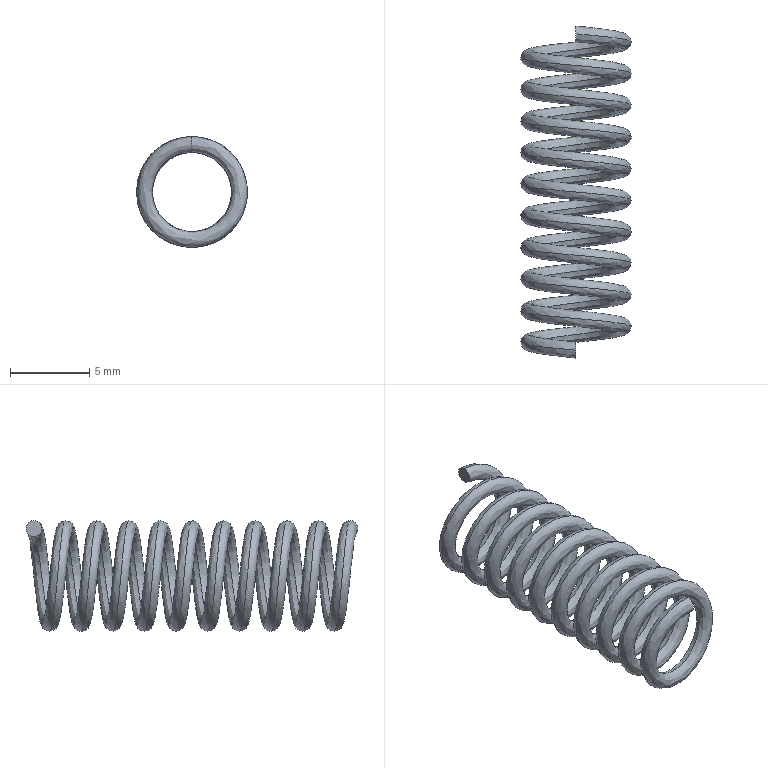Part | SolidWorks | features Helix 1, Sweep 1 | 1 solid | 4 faces | box 7 x 21 x 7 mm | volume 148.098 mm3 | spline 2 | plane 2